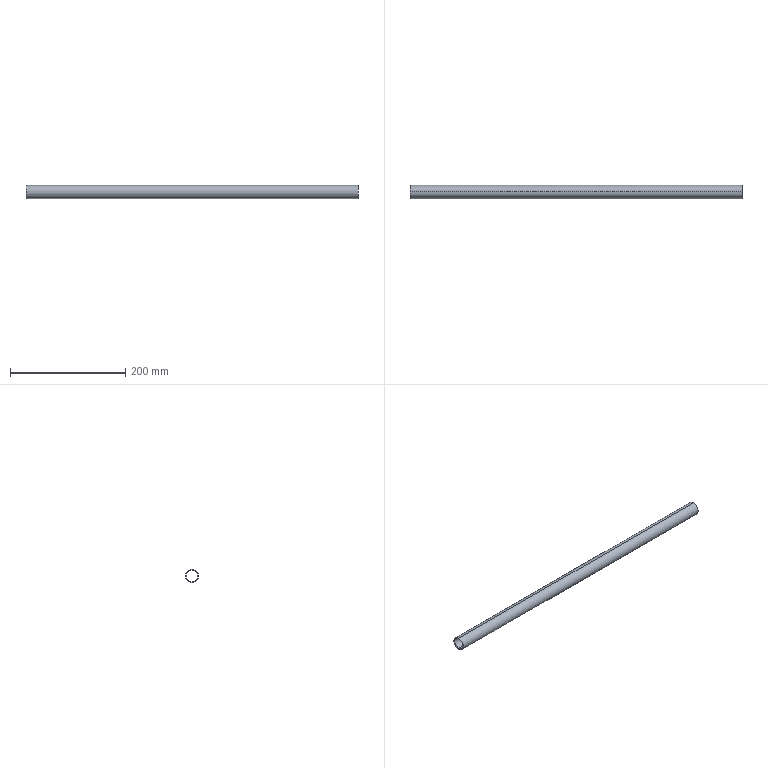Part | STEP file | 1 solid | 10 faces | box 576 x 23 x 23 mm | volume 58326 mm3 | cylinder 4 | cone 4 | plane 2 | commonest cylinder face diameters 20 x2 23 x2
STEP:
#1=CARTESIAN_POINT('',(0.,0.,0.));
#2=DIRECTION('',(0.,0.,1.));
#3=DIRECTION('',(1.,0.,0.));
#4=AXIS2_PLACEMENT_3D('',#1,#2,#3);
#5=CARTESIAN_POINT('',(576.,0.,11.5));
#6=VERTEX_POINT('',#5);
#7=CARTESIAN_POINT('',(576.,0.,-11.5));
#8=VERTEX_POINT('',#7);
#9=CARTESIAN_POINT('',(576.,0.,0.));
#10=DIRECTION('',(-1.,0.,0.));
#11=DIRECTION('',(0.,0.,1.));
#12=AXIS2_PLACEMENT_3D('',#9,#10,#11);
#13=CIRCLE('',#12,11.5);
#14=CARTESIAN_POINT('',(576.,0.,0.));
#15=DIRECTION('',(-1.,0.,0.));
#16=DIRECTION('',(0.,0.,1.));
#17=AXIS2_PLACEMENT_3D('',#14,#15,#16);
#18=CYLINDRICAL_SURFACE('',#17,11.5);
#19=CARTESIAN_POINT('',(0.,0.));
#20=DIRECTION('',(1.,0.));
#21=VECTOR('',#20,1.);
#22=LINE('',#19,#21);
#23=(GEOMETRIC_REPRESENTATION_CONTEXT(2)PARAMETRIC_REPRESENTATION_CONTEXT()REPRESENTATION_CONTEXT('',''));
#24=DEFINITIONAL_REPRESENTATION('',(#22),#23);
#25=PCURVE('',#18,#24);
#26=CARTESIAN_POINT('',(576.,10.707,0.));
#27=DIRECTION('',(-1.,0.,0.));
#28=DIRECTION('',(0.,0.,1.));
#29=AXIS2_PLACEMENT_3D('',#26,#27,#28);
#30=PLANE('',#29);
#31=CARTESIAN_POINT('',(0.,-10.707));
#32=DIRECTION('',(1.,0.));
#33=AXIS2_PLACEMENT_2D('',#31,#32);
#34=CIRCLE('',#33,11.5);
#35=(GEOMETRIC_REPRESENTATION_CONTEXT(2)PARAMETRIC_REPRESENTATION_CONTEXT()REPRESENTATION_CONTEXT('',''));
#36=DEFINITIONAL_REPRESENTATION('',(#34),#35);
#37=PCURVE('',#30,#36);
#38=SURFACE_CURVE('',#13,(#25,#37),.PCURVE_S1.);
#39=EDGE_CURVE('',#6,#8,#38,.T.);
#40=ORIENTED_EDGE('',*,*,#39,.T.);
#41=CARTESIAN_POINT('',(0.,0.,-11.5));
#42=VERTEX_POINT('',#41);
#43=CARTESIAN_POINT('',(576.,0.,-11.5));
#44=DIRECTION('',(-1.,0.,0.));
#45=VECTOR('',#44,1.);
#46=LINE('',#43,#45);
#47=CARTESIAN_POINT('',(3.142,0.));
#48=DIRECTION('',(0.,1.));
#49=VECTOR('',#48,1.);
#50=LINE('',#47,#49);
#51=(GEOMETRIC_REPRESENTATION_CONTEXT(2)PARAMETRIC_REPRESENTATION_CONTEXT()REPRESENTATION_CONTEXT('',''));
#52=DEFINITIONAL_REPRESENTATION('',(#50),#51);
#53=PCURVE('',#18,#52);
#54=CARTESIAN_POINT('',(576.,0.,0.));
#55=DIRECTION('',(-1.,0.,0.));
#56=DIRECTION('',(0.,0.,1.));
#57=AXIS2_PLACEMENT_3D('',#54,#55,#56);
#58=CYLINDRICAL_SURFACE('',#57,11.5);
#59=CARTESIAN_POINT('',(3.142,0.));
#60=DIRECTION('',(0.,1.));
#61=VECTOR('',#60,1.);
#62=LINE('',#59,#61);
#63=(GEOMETRIC_REPRESENTATION_CONTEXT(2)PARAMETRIC_REPRESENTATION_CONTEXT()REPRESENTATION_CONTEXT('',''));
#64=DEFINITIONAL_REPRESENTATION('',(#62),#63);
#65=PCURVE('',#58,#64);
#66=SURFACE_CURVE('',#46,(#53,#65),.PCURVE_S1.);
#67=EDGE_CURVE('',#8,#42,#66,.T.);
#68=ORIENTED_EDGE('',*,*,#67,.T.);
#69=CARTESIAN_POINT('',(0.,0.,11.5));
#70=VERTEX_POINT('',#69);
#71=CARTESIAN_POINT('',(0.,0.,0.));
#72=DIRECTION('',(-1.,0.,0.));
#73=DIRECTION('',(0.,0.,1.));
#74=AXIS2_PLACEMENT_3D('',#71,#72,#73);
#75=CIRCLE('',#74,11.5);
#76=CARTESIAN_POINT('',(0.,576.));
#77=DIRECTION('',(1.,0.));
#78=VECTOR('',#77,1.);
#79=LINE('',#76,#78);
#80=(GEOMETRIC_REPRESENTATION_CONTEXT(2)PARAMETRIC_REPRESENTATION_CONTEXT()REPRESENTATION_CONTEXT('',''));
#81=DEFINITIONAL_REPRESENTATION('',(#79),#80);
#82=PCURVE('',#18,#81);
#83=CARTESIAN_POINT('',(0.,11.5,0.));
#84=DIRECTION('',(1.,0.,0.));
#85=DIRECTION('',(0.,0.,-1.));
#86=AXIS2_PLACEMENT_3D('',#83,#84,#85);
#87=PLANE('',#86);
#88=CARTESIAN_POINT('',(-11.5,-11.5));
#89=CARTESIAN_POINT('',(-11.5,8.419));
#90=CARTESIAN_POINT('',(5.75,-1.541));
#91=CARTESIAN_POINT('',(23.,-11.5));
#92=CARTESIAN_POINT('',(5.75,-21.459));
#93=CARTESIAN_POINT('',(-11.5,-31.419));
#94=CARTESIAN_POINT('',(-11.5,-11.5));
#95=(BOUNDED_CURVE()B_SPLINE_CURVE(2,(#88,#89,#90,#91,#92,#93,#94),.UNSPECIFIED.,.T.,.F.)B_SPLINE_CURVE_WITH_KNOTS((1,2,2,2,2,1),(-2.094,0.,2.094,4.189,6.283,8.378),.UNSPECIFIED.)CURVE()GEOMETRIC_REPRESENTATION_ITEM()RATIONAL_B_SPLINE_CURVE((1.,0.5,1.,0.5,1.,0.5,1.))REPRESENTATION_ITEM(''));
#96=(GEOMETRIC_REPRESENTATION_CONTEXT(2)PARAMETRIC_REPRESENTATION_CONTEXT()REPRESENTATION_CONTEXT('',''));
#97=DEFINITIONAL_REPRESENTATION('',(#95),#96);
#98=PCURVE('',#87,#97);
#99=SURFACE_CURVE('',#75,(#82,#98),.PCURVE_S1.);
#100=EDGE_CURVE('',#70,#42,#99,.T.);
#101=ORIENTED_EDGE('',*,*,#100,.F.);
#102=CARTESIAN_POINT('',(576.,0.,11.5));
#103=DIRECTION('',(-1.,0.,0.));
#104=VECTOR('',#103,1.);
#105=LINE('',#102,#104);
#106=CARTESIAN_POINT('',(0.,0.));
#107=DIRECTION('',(0.,1.));
#108=VECTOR('',#107,1.);
#109=LINE('',#106,#108);
#110=(GEOMETRIC_REPRESENTATION_CONTEXT(2)PARAMETRIC_REPRESENTATION_CONTEXT()REPRESENTATION_CONTEXT('',''));
#111=DEFINITIONAL_REPRESENTATION('',(#109),#110);
#112=PCURVE('',#18,#111);
#113=CARTESIAN_POINT('',(6.283,0.));
#114=DIRECTION('',(0.,1.));
#115=VECTOR('',#114,1.);
#116=LINE('',#113,#115);
#117=(GEOMETRIC_REPRESENTATION_CONTEXT(2)PARAMETRIC_REPRESENTATION_CONTEXT()REPRESENTATION_CONTEXT('',''));
#118=DEFINITIONAL_REPRESENTATION('',(#116),#117);
#119=PCURVE('',#58,#118);
#120=SURFACE_CURVE('',#105,(#112,#119),.PCURVE_S1.);
#121=EDGE_CURVE('',#6,#70,#120,.T.);
#122=ORIENTED_EDGE('',*,*,#121,.F.);
#123=EDGE_LOOP('',(#40,#68,#101,#122));
#124=FACE_BOUND('',#123,.T.);
#125=ADVANCED_FACE('',(#124),#18,.T.);
#126=CARTESIAN_POINT('',(575.293,0.,-10.));
#127=VERTEX_POINT('',#126);
#128=CARTESIAN_POINT('',(576.,0.,-10.707));
#129=VERTEX_POINT('',#128);
#130=CARTESIAN_POINT('',(575.293,0.,-10.));
#131=DIRECTION('',(0.7071,0.,-0.7071));
#132=VECTOR('',#131,1.);
#133=LINE('',#130,#132);
#134=CARTESIAN_POINT('',(575.293,0.,0.));
#135=DIRECTION('',(1.,0.,0.));
#136=DIRECTION('',(0.,0.,-1.));
#137=AXIS2_PLACEMENT_3D('',#134,#135,#136);
#138=CONICAL_SURFACE('',#137,10.,0.7854);
#139=CARTESIAN_POINT('',(6.283,0.));
#140=DIRECTION('',(0.,1.));
#141=VECTOR('',#140,1.);
#142=LINE('',#139,#141);
#143=(GEOMETRIC_REPRESENTATION_CONTEXT(2)PARAMETRIC_REPRESENTATION_CONTEXT()REPRESENTATION_CONTEXT('',''));
#144=DEFINITIONAL_REPRESENTATION('',(#142),#143);
#145=PCURVE('',#138,#144);
#146=CARTESIAN_POINT('',(575.293,0.,0.));
#147=DIRECTION('',(1.,0.,0.));
#148=DIRECTION('',(0.,0.,-1.));
#149=AXIS2_PLACEMENT_3D('',#146,#147,#148);
#150=CONICAL_SURFACE('',#149,10.,0.7854);
#151=CARTESIAN_POINT('',(0.,0.));
#152=DIRECTION('',(0.,1.));
#153=VECTOR('',#152,1.);
#154=LINE('',#151,#153);
#155=(GEOMETRIC_REPRESENTATION_CONTEXT(2)PARAMETRIC_REPRESENTATION_CONTEXT()REPRESENTATION_CONTEXT('',''));
#156=DEFINITIONAL_REPRESENTATION('',(#154),#155);
#157=PCURVE('',#150,#156);
#158=SURFACE_CURVE('',#133,(#145,#157),.PCURVE_S1.);
#159=EDGE_CURVE('',#127,#129,#158,.T.);
#160=ORIENTED_EDGE('',*,*,#159,.T.);
#161=CARTESIAN_POINT('',(576.,0.,10.707));
#162=VERTEX_POINT('',#161);
#163=CARTESIAN_POINT('',(576.,0.,0.));
#164=DIRECTION('',(-1.,0.,0.));
#165=DIRECTION('',(0.,0.,1.));
#166=AXIS2_PLACEMENT_3D('',#163,#164,#165);
#167=CIRCLE('',#166,10.707);
#168=CARTESIAN_POINT('',(9.425,0.7071));
#169=DIRECTION('',(-1.,0.));
#170=VECTOR('',#169,1.);
#171=LINE('',#168,#170);
#172=(GEOMETRIC_REPRESENTATION_CONTEXT(2)PARAMETRIC_REPRESENTATION_CONTEXT()REPRESENTATION_CONTEXT('',''));
#173=DEFINITIONAL_REPRESENTATION('',(#171),#172);
#174=PCURVE('',#138,#173);
#175=CARTESIAN_POINT('',(0.,-10.707));
#176=DIRECTION('',(1.,0.));
#177=AXIS2_PLACEMENT_2D('',#175,#176);
#178=CIRCLE('',#177,10.707);
#179=(GEOMETRIC_REPRESENTATION_CONTEXT(2)PARAMETRIC_REPRESENTATION_CONTEXT()REPRESENTATION_CONTEXT('',''));
#180=DEFINITIONAL_REPRESENTATION('',(#178),#179);
#181=PCURVE('',#30,#180);
#182=SURFACE_CURVE('',#167,(#174,#181),.PCURVE_S1.);
#183=EDGE_CURVE('',#129,#162,#182,.T.);
#184=ORIENTED_EDGE('',*,*,#183,.T.);
#185=CARTESIAN_POINT('',(575.293,0.,10.));
#186=VERTEX_POINT('',#185);
#187=CARTESIAN_POINT('',(575.293,0.,10.));
#188=DIRECTION('',(0.7071,0.,0.7071));
#189=VECTOR('',#188,1.);
#190=LINE('',#187,#189);
#191=CARTESIAN_POINT('',(3.142,0.));
#192=DIRECTION('',(0.,1.));
#193=VECTOR('',#192,1.);
#194=LINE('',#191,#193);
#195=(GEOMETRIC_REPRESENTATION_CONTEXT(2)PARAMETRIC_REPRESENTATION_CONTEXT()REPRESENTATION_CONTEXT('',''));
#196=DEFINITIONAL_REPRESENTATION('',(#194),#195);
#197=PCURVE('',#138,#196);
#198=CARTESIAN_POINT('',(3.142,0.));
#199=DIRECTION('',(0.,1.));
#200=VECTOR('',#199,1.);
#201=LINE('',#198,#200);
#202=(GEOMETRIC_REPRESENTATION_CONTEXT(2)PARAMETRIC_REPRESENTATION_CONTEXT()REPRESENTATION_CONTEXT('',''));
#203=DEFINITIONAL_REPRESENTATION('',(#201),#202);
#204=PCURVE('',#150,#203);
#205=SURFACE_CURVE('',#190,(#197,#204),.PCURVE_S1.);
#206=EDGE_CURVE('',#186,#162,#205,.T.);
#207=ORIENTED_EDGE('',*,*,#206,.F.);
#208=CARTESIAN_POINT('',(575.293,0.,0.));
#209=DIRECTION('',(-1.,0.,0.));
#210=DIRECTION('',(0.,0.,1.));
#211=AXIS2_PLACEMENT_3D('',#208,#209,#210);
#212=CIRCLE('',#211,10.);
#213=CARTESIAN_POINT('',(9.425,0.));
#214=DIRECTION('',(-1.,0.));
#215=VECTOR('',#214,1.);
#216=LINE('',#213,#215);
#217=(GEOMETRIC_REPRESENTATION_CONTEXT(2)PARAMETRIC_REPRESENTATION_CONTEXT()REPRESENTATION_CONTEXT('',''));
#218=DEFINITIONAL_REPRESENTATION('',(#216),#217);
#219=PCURVE('',#138,#218);
#220=CARTESIAN_POINT('',(576.,0.,0.));
#221=DIRECTION('',(-1.,0.,0.));
#222=DIRECTION('',(0.,0.,1.));
#223=AXIS2_PLACEMENT_3D('',#220,#221,#222);
#224=CYLINDRICAL_SURFACE('',#223,10.);
#225=CARTESIAN_POINT('',(0.,0.7071));
#226=DIRECTION('',(1.,0.));
#227=VECTOR('',#226,1.);
#228=LINE('',#225,#227);
#229=(GEOMETRIC_REPRESENTATION_CONTEXT(2)PARAMETRIC_REPRESENTATION_CONTEXT()REPRESENTATION_CONTEXT('',''));
#230=DEFINITIONAL_REPRESENTATION('',(#228),#229);
#231=PCURVE('',#224,#230);
#232=SURFACE_CURVE('',#212,(#219,#231),.PCURVE_S1.);
#233=EDGE_CURVE('',#127,#186,#232,.T.);
#234=ORIENTED_EDGE('',*,*,#233,.F.);
#235=EDGE_LOOP('',(#160,#184,#207,#234));
#236=FACE_BOUND('',#235,.F.);
#237=ADVANCED_FACE('',(#236),#138,.F.);
#238=CARTESIAN_POINT('',(0.7071,0.,10.));
#239=VERTEX_POINT('',#238);
#240=CARTESIAN_POINT('',(576.,0.,10.));
#241=DIRECTION('',(-1.,0.,0.));
#242=VECTOR('',#241,1.);
#243=LINE('',#240,#242);
#244=CARTESIAN_POINT('',(6.283,0.));
#245=DIRECTION('',(0.,1.));
#246=VECTOR('',#245,1.);
#247=LINE('',#244,#246);
#248=(GEOMETRIC_REPRESENTATION_CONTEXT(2)PARAMETRIC_REPRESENTATION_CONTEXT()REPRESENTATION_CONTEXT('',''));
#249=DEFINITIONAL_REPRESENTATION('',(#247),#248);
#250=PCURVE('',#224,#249);
#251=CARTESIAN_POINT('',(576.,0.,0.));
#252=DIRECTION('',(-1.,0.,0.));
#253=DIRECTION('',(0.,0.,1.));
#254=AXIS2_PLACEMENT_3D('',#251,#252,#253);
#255=CYLINDRICAL_SURFACE('',#254,10.);
#256=CARTESIAN_POINT('',(0.,0.));
#257=DIRECTION('',(0.,1.));
#258=VECTOR('',#257,1.);
#259=LINE('',#256,#258);
#260=(GEOMETRIC_REPRESENTATION_CONTEXT(2)PARAMETRIC_REPRESENTATION_CONTEXT()REPRESENTATION_CONTEXT('',''));
#261=DEFINITIONAL_REPRESENTATION('',(#259),#260);
#262=PCURVE('',#255,#261);
#263=SURFACE_CURVE('',#243,(#250,#262),.PCURVE_S1.);
#264=EDGE_CURVE('',#186,#239,#263,.T.);
#265=ORIENTED_EDGE('',*,*,#264,.T.);
#266=CARTESIAN_POINT('',(0.7071,0.,-10.));
#267=VERTEX_POINT('',#266);
#268=CARTESIAN_POINT('',(0.7071,0.,0.));
#269=DIRECTION('',(-1.,0.,0.));
#270=DIRECTION('',(0.,0.,1.));
#271=AXIS2_PLACEMENT_3D('',#268,#269,#270);
#272=CIRCLE('',#271,10.);
#273=CARTESIAN_POINT('',(0.,575.293));
#274=DIRECTION('',(1.,0.));
#275=VECTOR('',#274,1.);
#276=LINE('',#273,#275);
#277=(GEOMETRIC_REPRESENTATION_CONTEXT(2)PARAMETRIC_REPRESENTATION_CONTEXT()REPRESENTATION_CONTEXT('',''));
#278=DEFINITIONAL_REPRESENTATION('',(#276),#277);
#279=PCURVE('',#224,#278);
#280=CARTESIAN_POINT('',(0.,0.,0.));
#281=DIRECTION('',(-1.,0.,0.));
#282=DIRECTION('',(0.,0.,1.));
#283=AXIS2_PLACEMENT_3D('',#280,#281,#282);
#284=CONICAL_SURFACE('',#283,10.707,0.7854);
#285=CARTESIAN_POINT('',(0.,-0.7071));
#286=DIRECTION('',(1.,0.));
#287=VECTOR('',#286,1.);
#288=LINE('',#285,#287);
#289=(GEOMETRIC_REPRESENTATION_CONTEXT(2)PARAMETRIC_REPRESENTATION_CONTEXT()REPRESENTATION_CONTEXT('',''));
#290=DEFINITIONAL_REPRESENTATION('',(#288),#289);
#291=PCURVE('',#284,#290);
#292=SURFACE_CURVE('',#272,(#279,#291),.PCURVE_S1.);
#293=EDGE_CURVE('',#267,#239,#292,.T.);
#294=ORIENTED_EDGE('',*,*,#293,.F.);
#295=CARTESIAN_POINT('',(576.,0.,-10.));
#296=DIRECTION('',(-1.,0.,0.));
#297=VECTOR('',#296,1.);
#298=LINE('',#295,#297);
#299=CARTESIAN_POINT('',(3.142,0.));
#300=DIRECTION('',(0.,1.));
#301=VECTOR('',#300,1.);
#302=LINE('',#299,#301);
#303=(GEOMETRIC_REPRESENTATION_CONTEXT(2)PARAMETRIC_REPRESENTATION_CONTEXT()REPRESENTATION_CONTEXT('',''));
#304=DEFINITIONAL_REPRESENTATION('',(#302),#303);
#305=PCURVE('',#224,#304);
#306=CARTESIAN_POINT('',(3.142,0.));
#307=DIRECTION('',(0.,1.));
#308=VECTOR('',#307,1.);
#309=LINE('',#306,#308);
#310=(GEOMETRIC_REPRESENTATION_CONTEXT(2)PARAMETRIC_REPRESENTATION_CONTEXT()REPRESENTATION_CONTEXT('',''));
#311=DEFINITIONAL_REPRESENTATION('',(#309),#310);
#312=PCURVE('',#255,#311);
#313=SURFACE_CURVE('',#298,(#305,#312),.PCURVE_S1.);
#314=EDGE_CURVE('',#127,#267,#313,.T.);
#315=ORIENTED_EDGE('',*,*,#314,.F.);
#316=ORIENTED_EDGE('',*,*,#233,.T.);
#317=EDGE_LOOP('',(#265,#294,#315,#316));
#318=FACE_BOUND('',#317,.F.);
#319=ADVANCED_FACE('',(#318),#224,.F.);
#320=CARTESIAN_POINT('',(0.,0.,10.707));
#321=VERTEX_POINT('',#320);
#322=CARTESIAN_POINT('',(0.,0.,10.707));
#323=DIRECTION('',(-0.7071,0.,0.7071));
#324=VECTOR('',#323,1.);
#325=LINE('',#322,#324);
#326=CARTESIAN_POINT('',(6.283,0.));
#327=DIRECTION('',(0.,1.));
#328=VECTOR('',#327,1.);
#329=LINE('',#326,#328);
#330=(GEOMETRIC_REPRESENTATION_CONTEXT(2)PARAMETRIC_REPRESENTATION_CONTEXT()REPRESENTATION_CONTEXT('',''));
#331=DEFINITIONAL_REPRESENTATION('',(#329),#330);
#332=PCURVE('',#284,#331);
#333=CARTESIAN_POINT('',(0.,0.,0.));
#334=DIRECTION('',(-1.,0.,0.));
#335=DIRECTION('',(0.,0.,1.));
#336=AXIS2_PLACEMENT_3D('',#333,#334,#335);
#337=CONICAL_SURFACE('',#336,10.707,0.7854);
#338=CARTESIAN_POINT('',(0.,0.));
#339=DIRECTION('',(0.,1.));
#340=VECTOR('',#339,1.);
#341=LINE('',#338,#340);
#342=(GEOMETRIC_REPRESENTATION_CONTEXT(2)PARAMETRIC_REPRESENTATION_CONTEXT()REPRESENTATION_CONTEXT('',''));
#343=DEFINITIONAL_REPRESENTATION('',(#341),#342);
#344=PCURVE('',#337,#343);
#345=SURFACE_CURVE('',#325,(#332,#344),.PCURVE_S1.);
#346=EDGE_CURVE('',#239,#321,#345,.T.);
#347=ORIENTED_EDGE('',*,*,#346,.T.);
#348=CARTESIAN_POINT('',(0.,0.,-10.707));
#349=VERTEX_POINT('',#348);
#350=CARTESIAN_POINT('',(0.,0.,0.));
#351=DIRECTION('',(-1.,0.,0.));
#352=DIRECTION('',(0.,0.,1.));
#353=AXIS2_PLACEMENT_3D('',#350,#351,#352);
#354=CIRCLE('',#353,10.707);
#355=CARTESIAN_POINT('',(0.,0.));
#356=DIRECTION('',(1.,0.));
#357=VECTOR('',#356,1.);
#358=LINE('',#355,#357);
#359=(GEOMETRIC_REPRESENTATION_CONTEXT(2)PARAMETRIC_REPRESENTATION_CONTEXT()REPRESENTATION_CONTEXT('',''));
#360=DEFINITIONAL_REPRESENTATION('',(#358),#359);
#361=PCURVE('',#284,#360);
#362=CARTESIAN_POINT('',(-10.707,-11.5));
#363=CARTESIAN_POINT('',(-10.707,7.045));
#364=CARTESIAN_POINT('',(5.354,-2.227));
#365=CARTESIAN_POINT('',(21.414,-11.5));
#366=CARTESIAN_POINT('',(5.354,-20.773));
#367=CARTESIAN_POINT('',(-10.707,-30.045));
#368=CARTESIAN_POINT('',(-10.707,-11.5));
#369=(BOUNDED_CURVE()B_SPLINE_CURVE(2,(#362,#363,#364,#365,#366,#367,#368),.UNSPECIFIED.,.T.,.F.)B_SPLINE_CURVE_WITH_KNOTS((1,2,2,2,2,1),(-2.094,0.,2.094,4.189,6.283,8.378),.UNSPECIFIED.)CURVE()GEOMETRIC_REPRESENTATION_ITEM()RATIONAL_B_SPLINE_CURVE((1.,0.5,1.,0.5,1.,0.5,1.))REPRESENTATION_ITEM(''));
#370=(GEOMETRIC_REPRESENTATION_CONTEXT(2)PARAMETRIC_REPRESENTATION_CONTEXT()REPRESENTATION_CONTEXT('',''));
#371=DEFINITIONAL_REPRESENTATION('',(#369),#370);
#372=PCURVE('',#87,#371);
#373=SURFACE_CURVE('',#354,(#361,#372),.PCURVE_S1.);
#374=EDGE_CURVE('',#349,#321,#373,.T.);
#375=ORIENTED_EDGE('',*,*,#374,.F.);
#376=CARTESIAN_POINT('',(0.,0.,-10.707));
#377=DIRECTION('',(-0.7071,0.,-0.7071));
#378=VECTOR('',#377,1.);
#379=LINE('',#376,#378);
#380=CARTESIAN_POINT('',(3.142,0.));
#381=DIRECTION('',(0.,1.));
#382=VECTOR('',#381,1.);
#383=LINE('',#380,#382);
#384=(GEOMETRIC_REPRESENTATION_CONTEXT(2)PARAMETRIC_REPRESENTATION_CONTEXT()REPRESENTATION_CONTEXT('',''));
#385=DEFINITIONAL_REPRESENTATION('',(#383),#384);
#386=PCURVE('',#284,#385);
#387=CARTESIAN_POINT('',(3.142,0.));
#388=DIRECTION('',(0.,1.));
#389=VECTOR('',#388,1.);
#390=LINE('',#387,#389);
#391=(GEOMETRIC_REPRESENTATION_CONTEXT(2)PARAMETRIC_REPRESENTATION_CONTEXT()REPRESENTATION_CONTEXT('',''));
#392=DEFINITIONAL_REPRESENTATION('',(#390),#391);
#393=PCURVE('',#337,#392);
#394=SURFACE_CURVE('',#379,(#386,#393),.PCURVE_S1.);
#395=EDGE_CURVE('',#267,#349,#394,.T.);
#396=ORIENTED_EDGE('',*,*,#395,.F.);
#397=ORIENTED_EDGE('',*,*,#293,.T.);
#398=EDGE_LOOP('',(#347,#375,#396,#397));
#399=FACE_BOUND('',#398,.F.);
#400=ADVANCED_FACE('',(#399),#284,.F.);
#401=CARTESIAN_POINT('',(0.,0.,0.));
#402=DIRECTION('',(-1.,0.,0.));
#403=DIRECTION('',(0.,0.,1.));
#404=AXIS2_PLACEMENT_3D('',#401,#402,#403);
#405=CIRCLE('',#404,10.707);
#406=CARTESIAN_POINT('',(-10.707,-11.5));
#407=CARTESIAN_POINT('',(-10.707,7.045));
#408=CARTESIAN_POINT('',(5.354,-2.227));
#409=CARTESIAN_POINT('',(21.414,-11.5));
#410=CARTESIAN_POINT('',(5.354,-20.773));
#411=CARTESIAN_POINT('',(-10.707,-30.045));
#412=CARTESIAN_POINT('',(-10.707,-11.5));
#413=(BOUNDED_CURVE()B_SPLINE_CURVE(2,(#406,#407,#408,#409,#410,#411,#412),.UNSPECIFIED.,.T.,.F.)B_SPLINE_CURVE_WITH_KNOTS((1,2,2,2,2,1),(-2.094,0.,2.094,4.189,6.283,8.378),.UNSPECIFIED.)CURVE()GEOMETRIC_REPRESENTATION_ITEM()RATIONAL_B_SPLINE_CURVE((1.,0.5,1.,0.5,1.,0.5,1.))REPRESENTATION_ITEM(''));
#414=(GEOMETRIC_REPRESENTATION_CONTEXT(2)PARAMETRIC_REPRESENTATION_CONTEXT()REPRESENTATION_CONTEXT('',''));
#415=DEFINITIONAL_REPRESENTATION('',(#413),#414);
#416=PCURVE('',#87,#415);
#417=CARTESIAN_POINT('',(0.,0.));
#418=DIRECTION('',(1.,0.));
#419=VECTOR('',#418,1.);
#420=LINE('',#417,#419);
#421=(GEOMETRIC_REPRESENTATION_CONTEXT(2)PARAMETRIC_REPRESENTATION_CONTEXT()REPRESENTATION_CONTEXT('',''));
#422=DEFINITIONAL_REPRESENTATION('',(#420),#421);
#423=PCURVE('',#337,#422);
#424=SURFACE_CURVE('',#405,(#416,#423),.PCURVE_S1.);
#425=EDGE_CURVE('',#321,#349,#424,.T.);
#426=ORIENTED_EDGE('',*,*,#425,.F.);
#427=ORIENTED_EDGE('',*,*,#374,.F.);
#428=EDGE_LOOP('',(#426,#427));
#429=FACE_BOUND('',#428,.T.);
#430=ORIENTED_EDGE('',*,*,#100,.T.);
#431=CARTESIAN_POINT('',(0.,0.,0.));
#432=DIRECTION('',(-1.,0.,0.));
#433=DIRECTION('',(0.,0.,1.));
#434=AXIS2_PLACEMENT_3D('',#431,#432,#433);
#435=CIRCLE('',#434,11.5);
#436=CARTESIAN_POINT('',(-11.5,-11.5));
#437=CARTESIAN_POINT('',(-11.5,8.419));
#438=CARTESIAN_POINT('',(5.75,-1.541));
#439=CARTESIAN_POINT('',(23.,-11.5));
#440=CARTESIAN_POINT('',(5.75,-21.459));
#441=CARTESIAN_POINT('',(-11.5,-31.419));
#442=CARTESIAN_POINT('',(-11.5,-11.5));
#443=(BOUNDED_CURVE()B_SPLINE_CURVE(2,(#436,#437,#438,#439,#440,#441,#442),.UNSPECIFIED.,.T.,.F.)B_SPLINE_CURVE_WITH_KNOTS((1,2,2,2,2,1),(-2.094,0.,2.094,4.189,6.283,8.378),.UNSPECIFIED.)CURVE()GEOMETRIC_REPRESENTATION_ITEM()RATIONAL_B_SPLINE_CURVE((1.,0.5,1.,0.5,1.,0.5,1.))REPRESENTATION_ITEM(''));
#444=(GEOMETRIC_REPRESENTATION_CONTEXT(2)PARAMETRIC_REPRESENTATION_CONTEXT()REPRESENTATION_CONTEXT('',''));
#445=DEFINITIONAL_REPRESENTATION('',(#443),#444);
#446=PCURVE('',#87,#445);
#447=CARTESIAN_POINT('',(0.,576.));
#448=DIRECTION('',(1.,0.));
#449=VECTOR('',#448,1.);
#450=LINE('',#447,#449);
#451=(GEOMETRIC_REPRESENTATION_CONTEXT(2)PARAMETRIC_REPRESENTATION_CONTEXT()REPRESENTATION_CONTEXT('',''));
#452=DEFINITIONAL_REPRESENTATION('',(#450),#451);
#453=PCURVE('',#58,#452);
#454=SURFACE_CURVE('',#435,(#446,#453),.PCURVE_S1.);
#455=EDGE_CURVE('',#42,#70,#454,.T.);
#456=ORIENTED_EDGE('',*,*,#455,.T.);
#457=EDGE_LOOP('',(#430,#456));
#458=FACE_BOUND('',#457,.T.);
#459=ADVANCED_FACE('',(#429,#458),#87,.F.);
#460=ORIENTED_EDGE('',*,*,#425,.F.);
#461=ORIENTED_EDGE('',*,*,#346,.F.);
#462=CARTESIAN_POINT('',(0.7071,0.,0.));
#463=DIRECTION('',(-1.,0.,0.));
#464=DIRECTION('',(0.,0.,1.));
#465=AXIS2_PLACEMENT_3D('',#462,#463,#464);
#466=CIRCLE('',#465,10.);
#467=CARTESIAN_POINT('',(0.,-0.7071));
#468=DIRECTION('',(1.,0.));
#469=VECTOR('',#468,1.);
#470=LINE('',#467,#469);
#471=(GEOMETRIC_REPRESENTATION_CONTEXT(2)PARAMETRIC_REPRESENTATION_CONTEXT()REPRESENTATION_CONTEXT('',''));
#472=DEFINITIONAL_REPRESENTATION('',(#470),#471);
#473=PCURVE('',#337,#472);
#474=CARTESIAN_POINT('',(0.,575.293));
#475=DIRECTION('',(1.,0.));
#476=VECTOR('',#475,1.);
#477=LINE('',#474,#476);
#478=(GEOMETRIC_REPRESENTATION_CONTEXT(2)PARAMETRIC_REPRESENTATION_CONTEXT()REPRESENTATION_CONTEXT('',''));
#479=DEFINITIONAL_REPRESENTATION('',(#477),#478);
#480=PCURVE('',#255,#479);
#481=SURFACE_CURVE('',#466,(#473,#480),.PCURVE_S1.);
#482=EDGE_CURVE('',#239,#267,#481,.T.);
#483=ORIENTED_EDGE('',*,*,#482,.T.);
#484=ORIENTED_EDGE('',*,*,#395,.T.);
#485=EDGE_LOOP('',(#460,#461,#483,#484));
#486=FACE_BOUND('',#485,.F.);
#487=ADVANCED_FACE('',(#486),#337,.F.);
#488=ORIENTED_EDGE('',*,*,#482,.F.);
#489=ORIENTED_EDGE('',*,*,#264,.F.);
#490=CARTESIAN_POINT('',(575.293,0.,0.));
#491=DIRECTION('',(-1.,0.,0.));
#492=DIRECTION('',(0.,0.,1.));
#493=AXIS2_PLACEMENT_3D('',#490,#491,#492);
#494=CIRCLE('',#493,10.);
#495=CARTESIAN_POINT('',(0.,0.7071));
#496=DIRECTION('',(1.,0.));
#497=VECTOR('',#496,1.);
#498=LINE('',#495,#497);
#499=(GEOMETRIC_REPRESENTATION_CONTEXT(2)PARAMETRIC_REPRESENTATION_CONTEXT()REPRESENTATION_CONTEXT('',''));
#500=DEFINITIONAL_REPRESENTATION('',(#498),#499);
#501=PCURVE('',#255,#500);
#502=CARTESIAN_POINT('',(3.142,0.));
#503=DIRECTION('',(-1.,0.));
#504=VECTOR('',#503,1.);
#505=LINE('',#502,#504);
#506=(GEOMETRIC_REPRESENTATION_CONTEXT(2)PARAMETRIC_REPRESENTATION_CONTEXT()REPRESENTATION_CONTEXT('',''));
#507=DEFINITIONAL_REPRESENTATION('',(#505),#506);
#508=PCURVE('',#150,#507);
#509=SURFACE_CURVE('',#494,(#501,#508),.PCURVE_S1.);
#510=EDGE_CURVE('',#186,#127,#509,.T.);
#511=ORIENTED_EDGE('',*,*,#510,.T.);
#512=ORIENTED_EDGE('',*,*,#314,.T.);
#513=EDGE_LOOP('',(#488,#489,#511,#512));
#514=FACE_BOUND('',#513,.F.);
#515=ADVANCED_FACE('',(#514),#255,.F.);
#516=CARTESIAN_POINT('',(576.,0.,0.));
#517=DIRECTION('',(-1.,0.,0.));
#518=DIRECTION('',(0.,0.,1.));
#519=AXIS2_PLACEMENT_3D('',#516,#517,#518);
#520=CIRCLE('',#519,10.707);
#521=CARTESIAN_POINT('',(3.142,0.7071));
#522=DIRECTION('',(-1.,0.));
#523=VECTOR('',#522,1.);
#524=LINE('',#521,#523);
#525=(GEOMETRIC_REPRESENTATION_CONTEXT(2)PARAMETRIC_REPRESENTATION_CONTEXT()REPRESENTATION_CONTEXT('',''));
#526=DEFINITIONAL_REPRESENTATION('',(#524),#525);
#527=PCURVE('',#150,#526);
#528=CARTESIAN_POINT('',(0.,-10.707));
#529=DIRECTION('',(1.,0.));
#530=AXIS2_PLACEMENT_2D('',#528,#529);
#531=CIRCLE('',#530,10.707);
#532=(GEOMETRIC_REPRESENTATION_CONTEXT(2)PARAMETRIC_REPRESENTATION_CONTEXT()REPRESENTATION_CONTEXT('',''));
#533=DEFINITIONAL_REPRESENTATION('',(#531),#532);
#534=PCURVE('',#30,#533);
#535=SURFACE_CURVE('',#520,(#527,#534),.PCURVE_S1.);
#536=EDGE_CURVE('',#162,#129,#535,.T.);
#537=ORIENTED_EDGE('',*,*,#536,.T.);
#538=ORIENTED_EDGE('',*,*,#159,.F.);
#539=ORIENTED_EDGE('',*,*,#510,.F.);
#540=ORIENTED_EDGE('',*,*,#206,.T.);
#541=EDGE_LOOP('',(#537,#538,#539,#540));
#542=FACE_BOUND('',#541,.F.);
#543=ADVANCED_FACE('',(#542),#150,.F.);
#544=ORIENTED_EDGE('',*,*,#39,.F.);
#545=CARTESIAN_POINT('',(576.,0.,0.));
#546=DIRECTION('',(-1.,0.,0.));
#547=DIRECTION('',(0.,0.,1.));
#548=AXIS2_PLACEMENT_3D('',#545,#546,#547);
#549=CIRCLE('',#548,11.5);
#550=CARTESIAN_POINT('',(0.,-10.707));
#551=DIRECTION('',(1.,0.));
#552=AXIS2_PLACEMENT_2D('',#550,#551);
#553=CIRCLE('',#552,11.5);
#554=(GEOMETRIC_REPRESENTATION_CONTEXT(2)PARAMETRIC_REPRESENTATION_CONTEXT()REPRESENTATION_CONTEXT('',''));
#555=DEFINITIONAL_REPRESENTATION('',(#553),#554);
#556=PCURVE('',#30,#555);
#557=CARTESIAN_POINT('',(0.,0.));
#558=DIRECTION('',(1.,0.));
#559=VECTOR('',#558,1.);
#560=LINE('',#557,#559);
#561=(GEOMETRIC_REPRESENTATION_CONTEXT(2)PARAMETRIC_REPRESENTATION_CONTEXT()REPRESENTATION_CONTEXT('',''));
#562=DEFINITIONAL_REPRESENTATION('',(#560),#561);
#563=PCURVE('',#58,#562);
#564=SURFACE_CURVE('',#549,(#556,#563),.PCURVE_S1.);
#565=EDGE_CURVE('',#8,#6,#564,.T.);
#566=ORIENTED_EDGE('',*,*,#565,.F.);
#567=EDGE_LOOP('',(#544,#566));
#568=FACE_BOUND('',#567,.T.);
#569=ORIENTED_EDGE('',*,*,#183,.T.);
#570=ORIENTED_EDGE('',*,*,#536,.T.);
#571=EDGE_LOOP('',(#569,#570));
#572=FACE_BOUND('',#571,.T.);
#573=ADVANCED_FACE('',(#568,#572),#30,.F.);
#574=ORIENTED_EDGE('',*,*,#67,.F.);
#575=ORIENTED_EDGE('',*,*,#565,.T.);
#576=ORIENTED_EDGE('',*,*,#121,.T.);
#577=ORIENTED_EDGE('',*,*,#455,.F.);
#578=EDGE_LOOP('',(#574,#575,#576,#577));
#579=FACE_BOUND('',#578,.T.);
#580=ADVANCED_FACE('',(#579),#58,.T.);
#581=CLOSED_SHELL('',(#125,#237,#319,#400,#459,#487,#515,#543,#573,#580));
#582=MANIFOLD_SOLID_BREP('',#581);
#583=(LENGTH_UNIT()NAMED_UNIT(*)SI_UNIT(.MILLI.,.METRE.));
#584=UNCERTAINTY_MEASURE_WITH_UNIT(LENGTH_MEASURE(0.0000001),#583,'','');
#585=(NAMED_UNIT(*)PLANE_ANGLE_UNIT()SI_UNIT($,.RADIAN.));
#586=(NAMED_UNIT(*)SI_UNIT($,.STERADIAN.)SOLID_ANGLE_UNIT());
#587=(GEOMETRIC_REPRESENTATION_CONTEXT(3)GLOBAL_UNCERTAINTY_ASSIGNED_CONTEXT((#584))GLOBAL_UNIT_ASSIGNED_CONTEXT((#583,#585,#586))REPRESENTATION_CONTEXT('',''));
#588=ADVANCED_BREP_SHAPE_REPRESENTATION('',(#4,#582),#587);